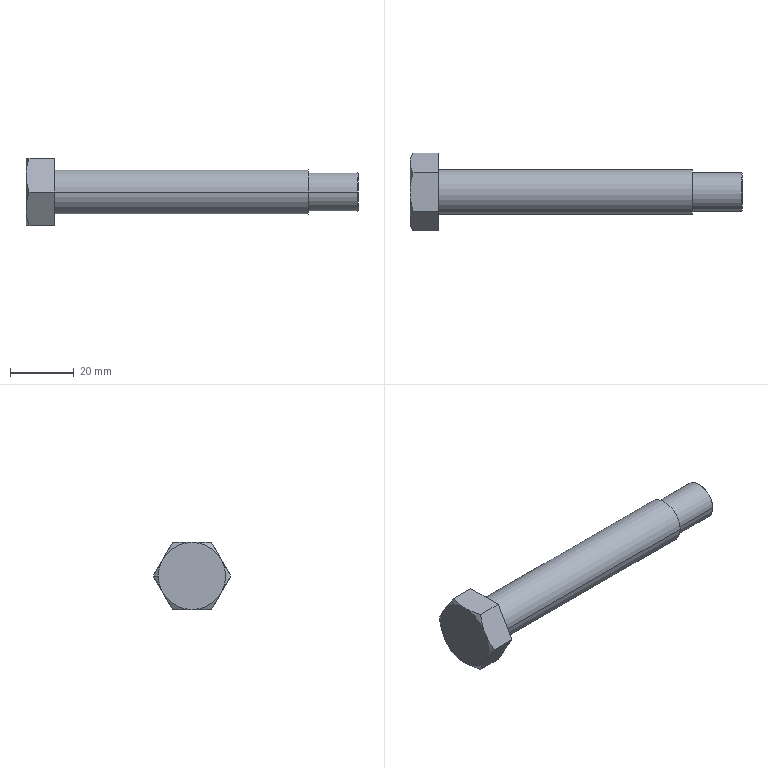Part | STEP file | PN_0025_M14x95 | 1 solid | 23 faces | box 103.8 x 24.249 x 21 mm | volume 17342 mm3 | plane 10 | cone 9 | cylinder 4 | commonest cylinder face diameters 12 x2 14 x2